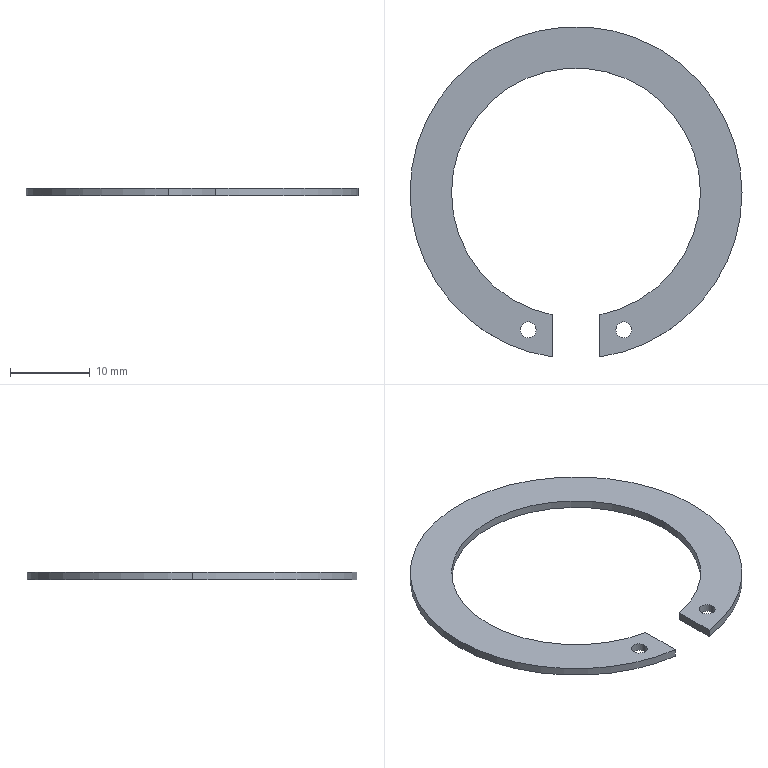Part | STEP file | Mkt rotor clip | 1 solid | 14 faces | box 41.6 x 41.383 x 1 mm | volume 557.011 mm3 | cylinder 10 | plane 4 | commonest cylinder face diameters 2 x4 31.2 x3 41.6 x3
STEP:
#1=CARTESIAN_POINT('',(0.,0.,0.));
#2=DIRECTION('',(0.,0.,1.));
#3=DIRECTION('',(1.,0.,0.));
#4=AXIS2_PLACEMENT_3D('',#1,#2,#3);
#5=CARTESIAN_POINT('',(5.,-17.2,1.));
#6=VERTEX_POINT('',#5);
#7=CARTESIAN_POINT('',(5.,-17.2,0.));
#8=VERTEX_POINT('',#7);
#9=CARTESIAN_POINT('',(5.,-17.2,1.));
#10=DIRECTION('',(0.,0.,-1.));
#11=VECTOR('',#10,1.);
#12=LINE('',#9,#11);
#13=CARTESIAN_POINT('',(6.,-17.2,1.));
#14=DIRECTION('',(0.,0.,-1.));
#15=DIRECTION('',(-1.,0.,0.));
#16=AXIS2_PLACEMENT_3D('',#13,#14,#15);
#17=CYLINDRICAL_SURFACE('',#16,1.);
#18=CARTESIAN_POINT('',(6.283,0.));
#19=DIRECTION('',(0.,1.));
#20=VECTOR('',#19,1.);
#21=LINE('',#18,#20);
#22=(GEOMETRIC_REPRESENTATION_CONTEXT(2)PARAMETRIC_REPRESENTATION_CONTEXT()REPRESENTATION_CONTEXT('',''));
#23=DEFINITIONAL_REPRESENTATION('',(#21),#22);
#24=PCURVE('',#17,#23);
#25=CARTESIAN_POINT('',(6.,-17.2,1.));
#26=DIRECTION('',(0.,0.,-1.));
#27=DIRECTION('',(-1.,0.,0.));
#28=AXIS2_PLACEMENT_3D('',#25,#26,#27);
#29=CYLINDRICAL_SURFACE('',#28,1.);
#30=CARTESIAN_POINT('',(0.,0.));
#31=DIRECTION('',(0.,1.));
#32=VECTOR('',#31,1.);
#33=LINE('',#30,#32);
#34=(GEOMETRIC_REPRESENTATION_CONTEXT(2)PARAMETRIC_REPRESENTATION_CONTEXT()REPRESENTATION_CONTEXT('',''));
#35=DEFINITIONAL_REPRESENTATION('',(#33),#34);
#36=PCURVE('',#29,#35);
#37=SURFACE_CURVE('',#12,(#24,#36),.PCURVE_S1.);
#38=EDGE_CURVE('',#6,#8,#37,.T.);
#39=ORIENTED_EDGE('',*,*,#38,.T.);
#40=CARTESIAN_POINT('',(7.,-17.2,0.));
#41=VERTEX_POINT('',#40);
#42=CARTESIAN_POINT('',(6.,-17.2,0.));
#43=DIRECTION('',(0.,0.,-1.));
#44=DIRECTION('',(-1.,0.,0.));
#45=AXIS2_PLACEMENT_3D('',#42,#43,#44);
#46=CIRCLE('',#45,1.);
#47=CARTESIAN_POINT('',(0.,1.));
#48=DIRECTION('',(1.,0.));
#49=VECTOR('',#48,1.);
#50=LINE('',#47,#49);
#51=(GEOMETRIC_REPRESENTATION_CONTEXT(2)PARAMETRIC_REPRESENTATION_CONTEXT()REPRESENTATION_CONTEXT('',''));
#52=DEFINITIONAL_REPRESENTATION('',(#50),#51);
#53=PCURVE('',#17,#52);
#54=CARTESIAN_POINT('',(0.,0.,0.));
#55=DIRECTION('',(0.,0.,1.));
#56=DIRECTION('',(1.,0.,0.));
#57=AXIS2_PLACEMENT_3D('',#54,#55,#56);
#58=PLANE('',#57);
#59=CARTESIAN_POINT('',(5.,-17.2));
#60=CARTESIAN_POINT('',(5.,-15.468));
#61=CARTESIAN_POINT('',(6.5,-16.334));
#62=CARTESIAN_POINT('',(8.,-17.2));
#63=CARTESIAN_POINT('',(6.5,-18.066));
#64=CARTESIAN_POINT('',(5.,-18.932));
#65=CARTESIAN_POINT('',(5.,-17.2));
#66=(BOUNDED_CURVE()B_SPLINE_CURVE(2,(#59,#60,#61,#62,#63,#64,#65),.UNSPECIFIED.,.T.,.F.)B_SPLINE_CURVE_WITH_KNOTS((1,2,2,2,2,1),(-2.094,0.,2.094,4.189,6.283,8.378),.UNSPECIFIED.)CURVE()GEOMETRIC_REPRESENTATION_ITEM()RATIONAL_B_SPLINE_CURVE((1.,0.5,1.,0.5,1.,0.5,1.))REPRESENTATION_ITEM(''));
#67=(GEOMETRIC_REPRESENTATION_CONTEXT(2)PARAMETRIC_REPRESENTATION_CONTEXT()REPRESENTATION_CONTEXT('',''));
#68=DEFINITIONAL_REPRESENTATION('',(#66),#67);
#69=PCURVE('',#58,#68);
#70=SURFACE_CURVE('',#46,(#53,#69),.PCURVE_S1.);
#71=EDGE_CURVE('',#41,#8,#70,.T.);
#72=ORIENTED_EDGE('',*,*,#71,.F.);
#73=CARTESIAN_POINT('',(7.,-17.2,1.));
#74=VERTEX_POINT('',#73);
#75=CARTESIAN_POINT('',(7.,-17.2,1.));
#76=DIRECTION('',(0.,0.,-1.));
#77=VECTOR('',#76,1.);
#78=LINE('',#75,#77);
#79=CARTESIAN_POINT('',(3.142,0.));
#80=DIRECTION('',(0.,1.));
#81=VECTOR('',#80,1.);
#82=LINE('',#79,#81);
#83=(GEOMETRIC_REPRESENTATION_CONTEXT(2)PARAMETRIC_REPRESENTATION_CONTEXT()REPRESENTATION_CONTEXT('',''));
#84=DEFINITIONAL_REPRESENTATION('',(#82),#83);
#85=PCURVE('',#17,#84);
#86=CARTESIAN_POINT('',(3.142,0.));
#87=DIRECTION('',(0.,1.));
#88=VECTOR('',#87,1.);
#89=LINE('',#86,#88);
#90=(GEOMETRIC_REPRESENTATION_CONTEXT(2)PARAMETRIC_REPRESENTATION_CONTEXT()REPRESENTATION_CONTEXT('',''));
#91=DEFINITIONAL_REPRESENTATION('',(#89),#90);
#92=PCURVE('',#29,#91);
#93=SURFACE_CURVE('',#78,(#85,#92),.PCURVE_S1.);
#94=EDGE_CURVE('',#74,#41,#93,.T.);
#95=ORIENTED_EDGE('',*,*,#94,.F.);
#96=CARTESIAN_POINT('',(6.,-17.2,1.));
#97=DIRECTION('',(0.,0.,-1.));
#98=DIRECTION('',(-1.,0.,0.));
#99=AXIS2_PLACEMENT_3D('',#96,#97,#98);
#100=CIRCLE('',#99,1.);
#101=CARTESIAN_POINT('',(0.,0.));
#102=DIRECTION('',(1.,0.));
#103=VECTOR('',#102,1.);
#104=LINE('',#101,#103);
#105=(GEOMETRIC_REPRESENTATION_CONTEXT(2)PARAMETRIC_REPRESENTATION_CONTEXT()REPRESENTATION_CONTEXT('',''));
#106=DEFINITIONAL_REPRESENTATION('',(#104),#105);
#107=PCURVE('',#17,#106);
#108=CARTESIAN_POINT('',(0.,0.,1.));
#109=DIRECTION('',(0.,0.,1.));
#110=DIRECTION('',(1.,0.,0.));
#111=AXIS2_PLACEMENT_3D('',#108,#109,#110);
#112=PLANE('',#111);
#113=CARTESIAN_POINT('',(5.,-17.2));
#114=CARTESIAN_POINT('',(5.,-15.468));
#115=CARTESIAN_POINT('',(6.5,-16.334));
#116=CARTESIAN_POINT('',(8.,-17.2));
#117=CARTESIAN_POINT('',(6.5,-18.066));
#118=CARTESIAN_POINT('',(5.,-18.932));
#119=CARTESIAN_POINT('',(5.,-17.2));
#120=(BOUNDED_CURVE()B_SPLINE_CURVE(2,(#113,#114,#115,#116,#117,#118,#119),.UNSPECIFIED.,.T.,.F.)B_SPLINE_CURVE_WITH_KNOTS((1,2,2,2,2,1),(-2.094,0.,2.094,4.189,6.283,8.378),.UNSPECIFIED.)CURVE()GEOMETRIC_REPRESENTATION_ITEM()RATIONAL_B_SPLINE_CURVE((1.,0.5,1.,0.5,1.,0.5,1.))REPRESENTATION_ITEM(''));
#121=(GEOMETRIC_REPRESENTATION_CONTEXT(2)PARAMETRIC_REPRESENTATION_CONTEXT()REPRESENTATION_CONTEXT('',''));
#122=DEFINITIONAL_REPRESENTATION('',(#120),#121);
#123=PCURVE('',#112,#122);
#124=SURFACE_CURVE('',#100,(#107,#123),.PCURVE_S1.);
#125=EDGE_CURVE('',#74,#6,#124,.T.);
#126=ORIENTED_EDGE('',*,*,#125,.T.);
#127=EDGE_LOOP('',(#39,#72,#95,#126));
#128=FACE_BOUND('',#127,.F.);
#129=ADVANCED_FACE('',(#128),#17,.F.);
#130=CARTESIAN_POINT('',(3.,-15.309,0.));
#131=VERTEX_POINT('',#130);
#132=CARTESIAN_POINT('',(3.,-15.309,1.));
#133=VERTEX_POINT('',#132);
#134=CARTESIAN_POINT('',(3.,-15.309,1.));
#135=DIRECTION('',(0.,0.,1.));
#136=VECTOR('',#135,1.);
#137=LINE('',#134,#136);
#138=CARTESIAN_POINT('',(0.,0.,1.));
#139=DIRECTION('',(0.,0.,-1.));
#140=DIRECTION('',(-1.,0.,0.));
#141=AXIS2_PLACEMENT_3D('',#138,#139,#140);
#142=CYLINDRICAL_SURFACE('',#141,15.6);
#143=CARTESIAN_POINT('',(4.519,0.));
#144=DIRECTION('',(0.,-1.));
#145=VECTOR('',#144,1.);
#146=LINE('',#143,#145);
#147=(GEOMETRIC_REPRESENTATION_CONTEXT(2)PARAMETRIC_REPRESENTATION_CONTEXT()REPRESENTATION_CONTEXT('',''));
#148=DEFINITIONAL_REPRESENTATION('',(#146),#147);
#149=PCURVE('',#142,#148);
#150=CARTESIAN_POINT('',(3.,-15.309,1.));
#151=DIRECTION('',(1.,0.,0.));
#152=DIRECTION('',(0.,0.,-1.));
#153=AXIS2_PLACEMENT_3D('',#150,#151,#152);
#154=PLANE('',#153);
#155=CARTESIAN_POINT('',(0.,0.));
#156=DIRECTION('',(-1.,0.));
#157=VECTOR('',#156,1.);
#158=LINE('',#155,#157);
#159=(GEOMETRIC_REPRESENTATION_CONTEXT(2)PARAMETRIC_REPRESENTATION_CONTEXT()REPRESENTATION_CONTEXT('',''));
#160=DEFINITIONAL_REPRESENTATION('',(#158),#159);
#161=PCURVE('',#154,#160);
#162=SURFACE_CURVE('',#137,(#149,#161),.PCURVE_S1.);
#163=EDGE_CURVE('',#131,#133,#162,.T.);
#164=ORIENTED_EDGE('',*,*,#163,.F.);
#165=CARTESIAN_POINT('',(15.6,0.,0.));
#166=VERTEX_POINT('',#165);
#167=CARTESIAN_POINT('',(0.,0.,0.));
#168=DIRECTION('',(0.,0.,-1.));
#169=DIRECTION('',(-1.,0.,0.));
#170=AXIS2_PLACEMENT_3D('',#167,#168,#169);
#171=CIRCLE('',#170,15.6);
#172=CARTESIAN_POINT('',(0.,1.));
#173=DIRECTION('',(1.,0.));
#174=VECTOR('',#173,1.);
#175=LINE('',#172,#174);
#176=(GEOMETRIC_REPRESENTATION_CONTEXT(2)PARAMETRIC_REPRESENTATION_CONTEXT()REPRESENTATION_CONTEXT('',''));
#177=DEFINITIONAL_REPRESENTATION('',(#175),#176);
#178=PCURVE('',#142,#177);
#179=CARTESIAN_POINT('',(-15.6,0.));
#180=CARTESIAN_POINT('',(-15.6,27.02));
#181=CARTESIAN_POINT('',(7.8,13.51));
#182=CARTESIAN_POINT('',(31.2,0.));
#183=CARTESIAN_POINT('',(7.8,-13.51));
#184=CARTESIAN_POINT('',(-15.6,-27.02));
#185=CARTESIAN_POINT('',(-15.6,0.));
#186=(BOUNDED_CURVE()B_SPLINE_CURVE(2,(#179,#180,#181,#182,#183,#184,#185),.UNSPECIFIED.,.T.,.F.)B_SPLINE_CURVE_WITH_KNOTS((1,2,2,2,2,1),(-2.094,0.,2.094,4.189,6.283,8.378),.UNSPECIFIED.)CURVE()GEOMETRIC_REPRESENTATION_ITEM()RATIONAL_B_SPLINE_CURVE((1.,0.5,1.,0.5,1.,0.5,1.))REPRESENTATION_ITEM(''));
#187=(GEOMETRIC_REPRESENTATION_CONTEXT(2)PARAMETRIC_REPRESENTATION_CONTEXT()REPRESENTATION_CONTEXT('',''));
#188=DEFINITIONAL_REPRESENTATION('',(#186),#187);
#189=PCURVE('',#58,#188);
#190=SURFACE_CURVE('',#171,(#178,#189),.PCURVE_S1.);
#191=EDGE_CURVE('',#166,#131,#190,.T.);
#192=ORIENTED_EDGE('',*,*,#191,.F.);
#193=CARTESIAN_POINT('',(15.6,0.,1.));
#194=VERTEX_POINT('',#193);
#195=CARTESIAN_POINT('',(15.6,0.,1.));
#196=DIRECTION('',(0.,0.,-1.));
#197=VECTOR('',#196,1.);
#198=LINE('',#195,#197);
#199=CARTESIAN_POINT('',(3.142,0.));
#200=DIRECTION('',(0.,1.));
#201=VECTOR('',#200,1.);
#202=LINE('',#199,#201);
#203=(GEOMETRIC_REPRESENTATION_CONTEXT(2)PARAMETRIC_REPRESENTATION_CONTEXT()REPRESENTATION_CONTEXT('',''));
#204=DEFINITIONAL_REPRESENTATION('',(#202),#203);
#205=PCURVE('',#142,#204);
#206=CARTESIAN_POINT('',(0.,0.,1.));
#207=DIRECTION('',(0.,0.,-1.));
#208=DIRECTION('',(-1.,0.,0.));
#209=AXIS2_PLACEMENT_3D('',#206,#207,#208);
#210=CYLINDRICAL_SURFACE('',#209,15.6);
#211=CARTESIAN_POINT('',(3.142,0.));
#212=DIRECTION('',(0.,1.));
#213=VECTOR('',#212,1.);
#214=LINE('',#211,#213);
#215=(GEOMETRIC_REPRESENTATION_CONTEXT(2)PARAMETRIC_REPRESENTATION_CONTEXT()REPRESENTATION_CONTEXT('',''));
#216=DEFINITIONAL_REPRESENTATION('',(#214),#215);
#217=PCURVE('',#210,#216);
#218=SURFACE_CURVE('',#198,(#205,#217),.PCURVE_S1.);
#219=EDGE_CURVE('',#194,#166,#218,.T.);
#220=ORIENTED_EDGE('',*,*,#219,.F.);
#221=CARTESIAN_POINT('',(0.,0.,1.));
#222=DIRECTION('',(0.,0.,-1.));
#223=DIRECTION('',(-1.,0.,0.));
#224=AXIS2_PLACEMENT_3D('',#221,#222,#223);
#225=CIRCLE('',#224,15.6);
#226=CARTESIAN_POINT('',(0.,0.));
#227=DIRECTION('',(1.,0.));
#228=VECTOR('',#227,1.);
#229=LINE('',#226,#228);
#230=(GEOMETRIC_REPRESENTATION_CONTEXT(2)PARAMETRIC_REPRESENTATION_CONTEXT()REPRESENTATION_CONTEXT('',''));
#231=DEFINITIONAL_REPRESENTATION('',(#229),#230);
#232=PCURVE('',#142,#231);
#233=CARTESIAN_POINT('',(-15.6,0.));
#234=CARTESIAN_POINT('',(-15.6,27.02));
#235=CARTESIAN_POINT('',(7.8,13.51));
#236=CARTESIAN_POINT('',(31.2,0.));
#237=CARTESIAN_POINT('',(7.8,-13.51));
#238=CARTESIAN_POINT('',(-15.6,-27.02));
#239=CARTESIAN_POINT('',(-15.6,0.));
#240=(BOUNDED_CURVE()B_SPLINE_CURVE(2,(#233,#234,#235,#236,#237,#238,#239),.UNSPECIFIED.,.T.,.F.)B_SPLINE_CURVE_WITH_KNOTS((1,2,2,2,2,1),(-2.094,0.,2.094,4.189,6.283,8.378),.UNSPECIFIED.)CURVE()GEOMETRIC_REPRESENTATION_ITEM()RATIONAL_B_SPLINE_CURVE((1.,0.5,1.,0.5,1.,0.5,1.))REPRESENTATION_ITEM(''));
#241=(GEOMETRIC_REPRESENTATION_CONTEXT(2)PARAMETRIC_REPRESENTATION_CONTEXT()REPRESENTATION_CONTEXT('',''));
#242=DEFINITIONAL_REPRESENTATION('',(#240),#241);
#243=PCURVE('',#112,#242);
#244=SURFACE_CURVE('',#225,(#232,#243),.PCURVE_S1.);
#245=EDGE_CURVE('',#194,#133,#244,.T.);
#246=ORIENTED_EDGE('',*,*,#245,.T.);
#247=EDGE_LOOP('',(#164,#192,#220,#246));
#248=FACE_BOUND('',#247,.F.);
#249=ADVANCED_FACE('',(#248),#142,.F.);
#250=CARTESIAN_POINT('',(-15.6,0.,0.));
#251=VERTEX_POINT('',#250);
#252=CARTESIAN_POINT('',(0.,0.,0.));
#253=DIRECTION('',(0.,0.,-1.));
#254=DIRECTION('',(-1.,0.,0.));
#255=AXIS2_PLACEMENT_3D('',#252,#253,#254);
#256=CIRCLE('',#255,15.6);
#257=CARTESIAN_POINT('',(0.,1.));
#258=DIRECTION('',(1.,0.));
#259=VECTOR('',#258,1.);
#260=LINE('',#257,#259);
#261=(GEOMETRIC_REPRESENTATION_CONTEXT(2)PARAMETRIC_REPRESENTATION_CONTEXT()REPRESENTATION_CONTEXT('',''));
#262=DEFINITIONAL_REPRESENTATION('',(#260),#261);
#263=PCURVE('',#210,#262);
#264=CARTESIAN_POINT('',(-15.6,0.));
#265=CARTESIAN_POINT('',(-15.6,27.02));
#266=CARTESIAN_POINT('',(7.8,13.51));
#267=CARTESIAN_POINT('',(31.2,0.));
#268=CARTESIAN_POINT('',(7.8,-13.51));
#269=CARTESIAN_POINT('',(-15.6,-27.02));
#270=CARTESIAN_POINT('',(-15.6,0.));
#271=(BOUNDED_CURVE()B_SPLINE_CURVE(2,(#264,#265,#266,#267,#268,#269,#270),.UNSPECIFIED.,.T.,.F.)B_SPLINE_CURVE_WITH_KNOTS((1,2,2,2,2,1),(-2.094,0.,2.094,4.189,6.283,8.378),.UNSPECIFIED.)CURVE()GEOMETRIC_REPRESENTATION_ITEM()RATIONAL_B_SPLINE_CURVE((1.,0.5,1.,0.5,1.,0.5,1.))REPRESENTATION_ITEM(''));
#272=(GEOMETRIC_REPRESENTATION_CONTEXT(2)PARAMETRIC_REPRESENTATION_CONTEXT()REPRESENTATION_CONTEXT('',''));
#273=DEFINITIONAL_REPRESENTATION('',(#271),#272);
#274=PCURVE('',#58,#273);
#275=SURFACE_CURVE('',#256,(#263,#274),.PCURVE_S1.);
#276=EDGE_CURVE('',#251,#166,#275,.T.);
#277=ORIENTED_EDGE('',*,*,#276,.F.);
#278=CARTESIAN_POINT('',(-15.6,0.,1.));
#279=VERTEX_POINT('',#278);
#280=CARTESIAN_POINT('',(-15.6,0.,1.));
#281=DIRECTION('',(0.,0.,-1.));
#282=VECTOR('',#281,1.);
#283=LINE('',#280,#282);
#284=CARTESIAN_POINT('',(0.,0.));
#285=DIRECTION('',(0.,1.));
#286=VECTOR('',#285,1.);
#287=LINE('',#284,#286);
#288=(GEOMETRIC_REPRESENTATION_CONTEXT(2)PARAMETRIC_REPRESENTATION_CONTEXT()REPRESENTATION_CONTEXT('',''));
#289=DEFINITIONAL_REPRESENTATION('',(#287),#288);
#290=PCURVE('',#210,#289);
#291=CARTESIAN_POINT('',(0.,0.,1.));
#292=DIRECTION('',(0.,0.,-1.));
#293=DIRECTION('',(-1.,0.,0.));
#294=AXIS2_PLACEMENT_3D('',#291,#292,#293);
#295=CYLINDRICAL_SURFACE('',#294,15.6);
#296=CARTESIAN_POINT('',(6.283,0.));
#297=DIRECTION('',(0.,1.));
#298=VECTOR('',#297,1.);
#299=LINE('',#296,#298);
#300=(GEOMETRIC_REPRESENTATION_CONTEXT(2)PARAMETRIC_REPRESENTATION_CONTEXT()REPRESENTATION_CONTEXT('',''));
#301=DEFINITIONAL_REPRESENTATION('',(#299),#300);
#302=PCURVE('',#295,#301);
#303=SURFACE_CURVE('',#283,(#290,#302),.PCURVE_S1.);
#304=EDGE_CURVE('',#279,#251,#303,.T.);
#305=ORIENTED_EDGE('',*,*,#304,.F.);
#306=CARTESIAN_POINT('',(0.,0.,1.));
#307=DIRECTION('',(0.,0.,-1.));
#308=DIRECTION('',(-1.,0.,0.));
#309=AXIS2_PLACEMENT_3D('',#306,#307,#308);
#310=CIRCLE('',#309,15.6);
#311=CARTESIAN_POINT('',(0.,0.));
#312=DIRECTION('',(1.,0.));
#313=VECTOR('',#312,1.);
#314=LINE('',#311,#313);
#315=(GEOMETRIC_REPRESENTATION_CONTEXT(2)PARAMETRIC_REPRESENTATION_CONTEXT()REPRESENTATION_CONTEXT('',''));
#316=DEFINITIONAL_REPRESENTATION('',(#314),#315);
#317=PCURVE('',#210,#316);
#318=CARTESIAN_POINT('',(-15.6,0.));
#319=CARTESIAN_POINT('',(-15.6,27.02));
#320=CARTESIAN_POINT('',(7.8,13.51));
#321=CARTESIAN_POINT('',(31.2,0.));
#322=CARTESIAN_POINT('',(7.8,-13.51));
#323=CARTESIAN_POINT('',(-15.6,-27.02));
#324=CARTESIAN_POINT('',(-15.6,0.));
#325=(BOUNDED_CURVE()B_SPLINE_CURVE(2,(#318,#319,#320,#321,#322,#323,#324),.UNSPECIFIED.,.T.,.F.)B_SPLINE_CURVE_WITH_KNOTS((1,2,2,2,2,1),(-2.094,0.,2.094,4.189,6.283,8.378),.UNSPECIFIED.)CURVE()GEOMETRIC_REPRESENTATION_ITEM()RATIONAL_B_SPLINE_CURVE((1.,0.5,1.,0.5,1.,0.5,1.))REPRESENTATION_ITEM(''));
#326=(GEOMETRIC_REPRESENTATION_CONTEXT(2)PARAMETRIC_REPRESENTATION_CONTEXT()REPRESENTATION_CONTEXT('',''));
#327=DEFINITIONAL_REPRESENTATION('',(#325),#326);
#328=PCURVE('',#112,#327);
#329=SURFACE_CURVE('',#310,(#317,#328),.PCURVE_S1.);
#330=EDGE_CURVE('',#279,#194,#329,.T.);
#331=ORIENTED_EDGE('',*,*,#330,.T.);
#332=ORIENTED_EDGE('',*,*,#219,.T.);
#333=EDGE_LOOP('',(#277,#305,#331,#332));
#334=FACE_BOUND('',#333,.F.);
#335=ADVANCED_FACE('',(#334),#210,.F.);
#336=CARTESIAN_POINT('',(-20.8,0.,1.));
#337=VERTEX_POINT('',#336);
#338=CARTESIAN_POINT('',(20.8,0.,1.));
#339=VERTEX_POINT('',#338);
#340=CARTESIAN_POINT('',(0.,0.,1.));
#341=DIRECTION('',(0.,0.,-1.));
#342=DIRECTION('',(-1.,0.,0.));
#343=AXIS2_PLACEMENT_3D('',#340,#341,#342);
#344=CIRCLE('',#343,20.8);
#345=CARTESIAN_POINT('',(0.,0.,1.));
#346=DIRECTION('',(0.,0.,-1.));
#347=DIRECTION('',(-1.,0.,0.));
#348=AXIS2_PLACEMENT_3D('',#345,#346,#347);
#349=CYLINDRICAL_SURFACE('',#348,20.8);
#350=CARTESIAN_POINT('',(0.,0.));
#351=DIRECTION('',(1.,0.));
#352=VECTOR('',#351,1.);
#353=LINE('',#350,#352);
#354=(GEOMETRIC_REPRESENTATION_CONTEXT(2)PARAMETRIC_REPRESENTATION_CONTEXT()REPRESENTATION_CONTEXT('',''));
#355=DEFINITIONAL_REPRESENTATION('',(#353),#354);
#356=PCURVE('',#349,#355);
#357=CARTESIAN_POINT('',(-20.8,0.));
#358=CARTESIAN_POINT('',(-20.8,36.027));
#359=CARTESIAN_POINT('',(10.4,18.013));
#360=CARTESIAN_POINT('',(41.6,0.));
#361=CARTESIAN_POINT('',(10.4,-18.013));
#362=CARTESIAN_POINT('',(-20.8,-36.027));
#363=CARTESIAN_POINT('',(-20.8,0.));
#364=(BOUNDED_CURVE()B_SPLINE_CURVE(2,(#357,#358,#359,#360,#361,#362,#363),.UNSPECIFIED.,.T.,.F.)B_SPLINE_CURVE_WITH_KNOTS((1,2,2,2,2,1),(-2.094,0.,2.094,4.189,6.283,8.378),.UNSPECIFIED.)CURVE()GEOMETRIC_REPRESENTATION_ITEM()RATIONAL_B_SPLINE_CURVE((1.,0.5,1.,0.5,1.,0.5,1.))REPRESENTATION_ITEM(''));
#365=(GEOMETRIC_REPRESENTATION_CONTEXT(2)PARAMETRIC_REPRESENTATION_CONTEXT()REPRESENTATION_CONTEXT('',''));
#366=DEFINITIONAL_REPRESENTATION('',(#364),#365);
#367=PCURVE('',#112,#366);
#368=SURFACE_CURVE('',#344,(#356,#367),.PCURVE_S1.);
#369=EDGE_CURVE('',#337,#339,#368,.T.);
#370=ORIENTED_EDGE('',*,*,#369,.T.);
#371=CARTESIAN_POINT('',(20.8,0.,0.));
#372=VERTEX_POINT('',#371);
#373=CARTESIAN_POINT('',(20.8,0.,1.));
#374=DIRECTION('',(0.,0.,-1.));
#375=VECTOR('',#374,1.);
#376=LINE('',#373,#375);
#377=CARTESIAN_POINT('',(3.142,0.));
#378=DIRECTION('',(0.,1.));
#379=VECTOR('',#378,1.);
#380=LINE('',#377,#379);
#381=(GEOMETRIC_REPRESENTATION_CONTEXT(2)PARAMETRIC_REPRESENTATION_CONTEXT()REPRESENTATION_CONTEXT('',''));
#382=DEFINITIONAL_REPRESENTATION('',(#380),#381);
#383=PCURVE('',#349,#382);
#384=CARTESIAN_POINT('',(0.,0.,1.));
#385=DIRECTION('',(0.,0.,-1.));
#386=DIRECTION('',(-1.,0.,0.));
#387=AXIS2_PLACEMENT_3D('',#384,#385,#386);
#388=CYLINDRICAL_SURFACE('',#387,20.8);
#389=CARTESIAN_POINT('',(3.142,0.));
#390=DIRECTION('',(0.,1.));
#391=VECTOR('',#390,1.);
#392=LINE('',#389,#391);
#393=(GEOMETRIC_REPRESENTATION_CONTEXT(2)PARAMETRIC_REPRESENTATION_CONTEXT()REPRESENTATION_CONTEXT('',''));
#394=DEFINITIONAL_REPRESENTATION('',(#392),#393);
#395=PCURVE('',#388,#394);
#396=SURFACE_CURVE('',#376,(#383,#395),.PCURVE_S1.);
#397=EDGE_CURVE('',#339,#372,#396,.T.);
#398=ORIENTED_EDGE('',*,*,#397,.T.);
#399=CARTESIAN_POINT('',(-20.8,0.,0.));
#400=VERTEX_POINT('',#399);
#401=CARTESIAN_POINT('',(0.,0.,0.));
#402=DIRECTION('',(0.,0.,1.));
#403=DIRECTION('',(-1.,0.,0.));
#404=AXIS2_PLACEMENT_3D('',#401,#402,#403);
#405=CIRCLE('',#404,20.8);
#406=CARTESIAN_POINT('',(6.283,1.));
#407=DIRECTION('',(-1.,0.));
#408=VECTOR('',#407,1.);
#409=LINE('',#406,#408);
#410=(GEOMETRIC_REPRESENTATION_CONTEXT(2)PARAMETRIC_REPRESENTATION_CONTEXT()REPRESENTATION_CONTEXT('',''));
#411=DEFINITIONAL_REPRESENTATION('',(#409),#410);
#412=PCURVE('',#349,#411);
#413=CARTESIAN_POINT('',(0.,0.));
#414=DIRECTION('',(-1.,0.));
#415=AXIS2_PLACEMENT_2D('',#413,#414);
#416=CIRCLE('',#415,20.8);
#417=(GEOMETRIC_REPRESENTATION_CONTEXT(2)PARAMETRIC_REPRESENTATION_CONTEXT()REPRESENTATION_CONTEXT('',''));
#418=DEFINITIONAL_REPRESENTATION('',(#416),#417);
#419=PCURVE('',#58,#418);
#420=SURFACE_CURVE('',#405,(#412,#419),.PCURVE_S1.);
#421=EDGE_CURVE('',#372,#400,#420,.T.);
#422=ORIENTED_EDGE('',*,*,#421,.T.);
#423=CARTESIAN_POINT('',(-20.8,0.,1.));
#424=DIRECTION('',(0.,0.,-1.));
#425=VECTOR('',#424,1.);
#426=LINE('',#423,#425);
#427=CARTESIAN_POINT('',(0.,0.));
#428=DIRECTION('',(0.,1.));
#429=VECTOR('',#428,1.);
#430=LINE('',#427,#429);
#431=(GEOMETRIC_REPRESENTATION_CONTEXT(2)PARAMETRIC_REPRESENTATION_CONTEXT()REPRESENTATION_CONTEXT('',''));
#432=DEFINITIONAL_REPRESENTATION('',(#430),#431);
#433=PCURVE('',#349,#432);
#434=CARTESIAN_POINT('',(0.,0.,1.));
#435=DIRECTION('',(0.,0.,-1.));
#436=DIRECTION('',(-1.,0.,0.));
#437=AXIS2_PLACEMENT_3D('',#434,#435,#436);
#438=CYLINDRICAL_SURFACE('',#437,20.8);
#439=CARTESIAN_POINT('',(6.283,0.));
#440=DIRECTION('',(0.,1.));
#441=VECTOR('',#440,1.);
#442=LINE('',#439,#441);
#443=(GEOMETRIC_REPRESENTATION_CONTEXT(2)PARAMETRIC_REPRESENTATION_CONTEXT()REPRESENTATION_CONTEXT('',''));
#444=DEFINITIONAL_REPRESENTATION('',(#442),#443);
#445=PCURVE('',#438,#444);
#446=SURFACE_CURVE('',#426,(#433,#445),.PCURVE_S1.);
#447=EDGE_CURVE('',#337,#400,#446,.T.);
#448=ORIENTED_EDGE('',*,*,#447,.F.);
#449=EDGE_LOOP('',(#370,#398,#422,#448));
#450=FACE_BOUND('',#449,.T.);
#451=ADVANCED_FACE('',(#450),#349,.T.);
#452=CARTESIAN_POINT('',(-3.,-20.583,1.));
#453=VERTEX_POINT('',#452);
#454=CARTESIAN_POINT('',(0.,0.,1.));
#455=DIRECTION('',(0.,0.,-1.));
#456=DIRECTION('',(-1.,0.,0.));
#457=AXIS2_PLACEMENT_3D('',#454,#455,#456);
#458=CIRCLE('',#457,20.8);
#459=CARTESIAN_POINT('',(0.,0.));
#460=DIRECTION('',(1.,0.));
#461=VECTOR('',#460,1.);
#462=LINE('',#459,#461);
#463=(GEOMETRIC_REPRESENTATION_CONTEXT(2)PARAMETRIC_REPRESENTATION_CONTEXT()REPRESENTATION_CONTEXT('',''));
#464=DEFINITIONAL_REPRESENTATION('',(#462),#463);
#465=PCURVE('',#438,#464);
#466=CARTESIAN_POINT('',(-20.8,0.));
#467=CARTESIAN_POINT('',(-20.8,36.027));
#468=CARTESIAN_POINT('',(10.4,18.013));
#469=CARTESIAN_POINT('',(41.6,0.));
#470=CARTESIAN_POINT('',(10.4,-18.013));
#471=CARTESIAN_POINT('',(-20.8,-36.027));
#472=CARTESIAN_POINT('',(-20.8,0.));
#473=(BOUNDED_CURVE()B_SPLINE_CURVE(2,(#466,#467,#468,#469,#470,#471,#472),.UNSPECIFIED.,.T.,.F.)B_SPLINE_CURVE_WITH_KNOTS((1,2,2,2,2,1),(-2.094,0.,2.094,4.189,6.283,8.378),.UNSPECIFIED.)CURVE()GEOMETRIC_REPRESENTATION_ITEM()RATIONAL_B_SPLINE_CURVE((1.,0.5,1.,0.5,1.,0.5,1.))REPRESENTATION_ITEM(''));
#474=(GEOMETRIC_REPRESENTATION_CONTEXT(2)PARAMETRIC_REPRESENTATION_CONTEXT()REPRESENTATION_CONTEXT('',''));
#475=DEFINITIONAL_REPRESENTATION('',(#473),#474);
#476=PCURVE('',#112,#475);
#477=SURFACE_CURVE('',#458,(#465,#476),.PCURVE_S1.);
#478=EDGE_CURVE('',#453,#337,#477,.T.);
#479=ORIENTED_EDGE('',*,*,#478,.T.);
#480=ORIENTED_EDGE('',*,*,#447,.T.);
#481=CARTESIAN_POINT('',(-3.,-20.583,0.));
#482=VERTEX_POINT('',#481);
#483=CARTESIAN_POINT('',(0.,0.,0.));
#484=DIRECTION('',(0.,0.,1.));
#485=DIRECTION('',(-1.,0.,0.));
#486=AXIS2_PLACEMENT_3D('',#483,#484,#485);
#487=CIRCLE('',#486,20.8);
#488=CARTESIAN_POINT('',(6.283,1.));
#489=DIRECTION('',(-1.,0.));
#490=VECTOR('',#489,1.);
#491=LINE('',#488,#490);
#492=(GEOMETRIC_REPRESENTATION_CONTEXT(2)PARAMETRIC_REPRESENTATION_CONTEXT()REPRESENTATION_CONTEXT('',''));
#493=DEFINITIONAL_REPRESENTATION('',(#491),#492);
#494=PCURVE('',#438,#493);
#495=CARTESIAN_POINT('',(0.,0.));
#496=DIRECTION('',(-1.,0.));
#497=AXIS2_PLACEMENT_2D('',#495,#496);
#498=CIRCLE('',#497,20.8);
#499=(GEOMETRIC_REPRESENTATION_CONTEXT(2)PARAMETRIC_REPRESENTATION_CONTEXT()REPRESENTATION_CONTEXT('',''));
#500=DEFINITIONAL_REPRESENTATION('',(#498),#499);
#501=PCURVE('',#58,#500);
#502=SURFACE_CURVE('',#487,(#494,#501),.PCURVE_S1.);
#503=EDGE_CURVE('',#400,#482,#502,.T.);
#504=ORIENTED_EDGE('',*,*,#503,.T.);
#505=CARTESIAN_POINT('',(-3.,-20.583,1.));
#506=DIRECTION('',(0.,0.,1.));
#507=VECTOR('',#506,1.);
#508=LINE('',#505,#507);
#509=CARTESIAN_POINT('',(4.857,0.));
#510=DIRECTION('',(0.,-1.));
#511=VECTOR('',#510,1.);
#512=LINE('',#509,#511);
#513=(GEOMETRIC_REPRESENTATION_CONTEXT(2)PARAMETRIC_REPRESENTATION_CONTEXT()REPRESENTATION_CONTEXT('',''));
#514=DEFINITIONAL_REPRESENTATION('',(#512),#513);
#515=PCURVE('',#438,#514);
#516=CARTESIAN_POINT('',(-3.,-15.309,1.));
#517=DIRECTION('',(-1.,0.,0.));
#518=DIRECTION('',(0.,0.,1.));
#519=AXIS2_PLACEMENT_3D('',#516,#517,#518);
#520=PLANE('',#519);
#521=CARTESIAN_POINT('',(0.,-5.274));
#522=DIRECTION('',(1.,0.));
#523=VECTOR('',#522,1.);
#524=LINE('',#521,#523);
#525=(GEOMETRIC_REPRESENTATION_CONTEXT(2)PARAMETRIC_REPRESENTATION_CONTEXT()REPRESENTATION_CONTEXT('',''));
#526=DEFINITIONAL_REPRESENTATION('',(#524),#525);
#527=PCURVE('',#520,#526);
#528=SURFACE_CURVE('',#508,(#515,#527),.PCURVE_S1.);
#529=EDGE_CURVE('',#482,#453,#528,.T.);
#530=ORIENTED_EDGE('',*,*,#529,.T.);
#531=EDGE_LOOP('',(#479,#480,#504,#530));
#532=FACE_BOUND('',#531,.T.);
#533=ADVANCED_FACE('',(#532),#438,.T.);
#534=CARTESIAN_POINT('',(-7.,-17.2,1.));
#535=VERTEX_POINT('',#534);
#536=CARTESIAN_POINT('',(-7.,-17.2,0.));
#537=VERTEX_POINT('',#536);
#538=CARTESIAN_POINT('',(-7.,-17.2,1.));
#539=DIRECTION('',(0.,0.,-1.));
#540=VECTOR('',#539,1.);
#541=LINE('',#538,#540);
#542=CARTESIAN_POINT('',(-6.,-17.2,1.));
#543=DIRECTION('',(0.,0.,-1.));
#544=DIRECTION('',(-1.,0.,0.));
#545=AXIS2_PLACEMENT_3D('',#542,#543,#544);
#546=CYLINDRICAL_SURFACE('',#545,1.);
#547=CARTESIAN_POINT('',(6.283,0.));
#548=DIRECTION('',(0.,1.));
#549=VECTOR('',#548,1.);
#550=LINE('',#547,#549);
#551=(GEOMETRIC_REPRESENTATION_CONTEXT(2)PARAMETRIC_REPRESENTATION_CONTEXT()REPRESENTATION_CONTEXT('',''));
#552=DEFINITIONAL_REPRESENTATION('',(#550),#551);
#553=PCURVE('',#546,#552);
#554=CARTESIAN_POINT('',(-6.,-17.2,1.));
#555=DIRECTION('',(0.,0.,-1.));
#556=DIRECTION('',(-1.,0.,0.));
#557=AXIS2_PLACEMENT_3D('',#554,#555,#556);
#558=CYLINDRICAL_SURFACE('',#557,1.);
#559=CARTESIAN_POINT('',(0.,0.));
#560=DIRECTION('',(0.,1.));
#561=VECTOR('',#560,1.);
#562=LINE('',#559,#561);
#563=(GEOMETRIC_REPRESENTATION_CONTEXT(2)PARAMETRIC_REPRESENTATION_CONTEXT()REPRESENTATION_CONTEXT('',''));
#564=DEFINITIONAL_REPRESENTATION('',(#562),#563);
#565=PCURVE('',#558,#564);
#566=SURFACE_CURVE('',#541,(#553,#565),.PCURVE_S1.);
#567=EDGE_CURVE('',#535,#537,#566,.T.);
#568=ORIENTED_EDGE('',*,*,#567,.T.);
#569=CARTESIAN_POINT('',(-5.,-17.2,0.));
#570=VERTEX_POINT('',#569);
#571=CARTESIAN_POINT('',(-6.,-17.2,0.));
#572=DIRECTION('',(0.,0.,-1.));
#573=DIRECTION('',(-1.,0.,0.));
#574=AXIS2_PLACEMENT_3D('',#571,#572,#573);
#575=CIRCLE('',#574,1.);
#576=CARTESIAN_POINT('',(0.,1.));
#577=DIRECTION('',(1.,0.));
#578=VECTOR('',#577,1.);
#579=LINE('',#576,#578);
#580=(GEOMETRIC_REPRESENTATION_CONTEXT(2)PARAMETRIC_REPRESENTATION_CONTEXT()REPRESENTATION_CONTEXT('',''));
#581=DEFINITIONAL_REPRESENTATION('',(#579),#580);
#582=PCURVE('',#546,#581);
#583=CARTESIAN_POINT('',(-7.,-17.2));
#584=CARTESIAN_POINT('',(-7.,-15.468));
#585=CARTESIAN_POINT('',(-5.5,-16.334));
#586=CARTESIAN_POINT('',(-4.,-17.2));
#587=CARTESIAN_POINT('',(-5.5,-18.066));
#588=CARTESIAN_POINT('',(-7.,-18.932));
#589=CARTESIAN_POINT('',(-7.,-17.2));
#590=(BOUNDED_CURVE()B_SPLINE_CURVE(2,(#583,#584,#585,#586,#587,#588,#589),.UNSPECIFIED.,.T.,.F.)B_SPLINE_CURVE_WITH_KNOTS((1,2,2,2,2,1),(-2.094,0.,2.094,4.189,6.283,8.378),.UNSPECIFIED.)CURVE()GEOMETRIC_REPRESENTATION_ITEM()RATIONAL_B_SPLINE_CURVE((1.,0.5,1.,0.5,1.,0.5,1.))REPRESENTATION_ITEM(''));
#591=(GEOMETRIC_REPRESENTATION_CONTEXT(2)PARAMETRIC_REPRESENTATION_CONTEXT()REPRESENTATION_CONTEXT('',''));
#592=DEFINITIONAL_REPRESENTATION('',(#590),#591);
#593=PCURVE('',#58,#592);
#594=SURFACE_CURVE('',#575,(#582,#593),.PCURVE_S1.);
#595=EDGE_CURVE('',#570,#537,#594,.T.);
#596=ORIENTED_EDGE('',*,*,#595,.F.);
#597=CARTESIAN_POINT('',(-5.,-17.2,1.));
#598=VERTEX_POINT('',#597);
#599=CARTESIAN_POINT('',(-5.,-17.2,1.));
#600=DIRECTION('',(0.,0.,-1.));
#601=VECTOR('',#600,1.);
#602=LINE('',#599,#601);
#603=CARTESIAN_POINT('',(3.142,0.));
#604=DIRECTION('',(0.,1.));
#605=VECTOR('',#604,1.);
#606=LINE('',#603,#605);
#607=(GEOMETRIC_REPRESENTATION_CONTEXT(2)PARAMETRIC_REPRESENTATION_CONTEXT()REPRESENTATION_CONTEXT('',''));
#608=DEFINITIONAL_REPRESENTATION('',(#606),#607);
#609=PCURVE('',#546,#608);
#610=CARTESIAN_POINT('',(3.142,0.));
#611=DIRECTION('',(0.,1.));
#612=VECTOR('',#611,1.);
#613=LINE('',#610,#612);
#614=(GEOMETRIC_REPRESENTATION_CONTEXT(2)PARAMETRIC_REPRESENTATION_CONTEXT()REPRESENTATION_CONTEXT('',''));
#615=DEFINITIONAL_REPRESENTATION('',(#613),#614);
#616=PCURVE('',#558,#615);
#617=SURFACE_CURVE('',#602,(#609,#616),.PCURVE_S1.);
#618=EDGE_CURVE('',#598,#570,#617,.T.);
#619=ORIENTED_EDGE('',*,*,#618,.F.);
#620=CARTESIAN_POINT('',(-6.,-17.2,1.));
#621=DIRECTION('',(0.,0.,-1.));
#622=DIRECTION('',(-1.,0.,0.));
#623=AXIS2_PLACEMENT_3D('',#620,#621,#622);
#624=CIRCLE('',#623,1.);
#625=CARTESIAN_POINT('',(0.,0.));
#626=DIRECTION('',(1.,0.));
#627=VECTOR('',#626,1.);
#628=LINE('',#625,#627);
#629=(GEOMETRIC_REPRESENTATION_CONTEXT(2)PARAMETRIC_REPRESENTATION_CONTEXT()REPRESENTATION_CONTEXT('',''));
#630=DEFINITIONAL_REPRESENTATION('',(#628),#629);
#631=PCURVE('',#546,#630);
#632=CARTESIAN_POINT('',(-7.,-17.2));
#633=CARTESIAN_POINT('',(-7.,-15.468));
#634=CARTESIAN_POINT('',(-5.5,-16.334));
#635=CARTESIAN_POINT('',(-4.,-17.2));
#636=CARTESIAN_POINT('',(-5.5,-18.066));
#637=CARTESIAN_POINT('',(-7.,-18.932));
#638=CARTESIAN_POINT('',(-7.,-17.2));
#639=(BOUNDED_CURVE()B_SPLINE_CURVE(2,(#632,#633,#634,#635,#636,#637,#638),.UNSPECIFIED.,.T.,.F.)B_SPLINE_CURVE_WITH_KNOTS((1,2,2,2,2,1),(-2.094,0.,2.094,4.189,6.283,8.378),.UNSPECIFIED.)CURVE()GEOMETRIC_REPRESENTATION_ITEM()RATIONAL_B_SPLINE_CURVE((1.,0.5,1.,0.5,1.,0.5,1.))REPRESENTATION_ITEM(''));
#640=(GEOMETRIC_REPRESENTATION_CONTEXT(2)PARAMETRIC_REPRESENTATION_CONTEXT()REPRESENTATION_CONTEXT('',''));
#641=DEFINITIONAL_REPRESENTATION('',(#639),#640);
#642=PCURVE('',#112,#641);
#643=SURFACE_CURVE('',#624,(#631,#642),.PCURVE_S1.);
#644=EDGE_CURVE('',#598,#535,#643,.T.);
#645=ORIENTED_EDGE('',*,*,#644,.T.);
#646=EDGE_LOOP('',(#568,#596,#619,#645));
#647=FACE_BOUND('',#646,.F.);
#648=ADVANCED_FACE('',(#647),#546,.F.);
#649=CARTESIAN_POINT('',(6.,-17.2,0.));
#650=DIRECTION('',(0.,0.,-1.));
#651=DIRECTION('',(-1.,0.,0.));
#652=AXIS2_PLACEMENT_3D('',#649,#650,#651);
#653=CIRCLE('',#652,1.);
#654=CARTESIAN_POINT('',(5.,-17.2));
#655=CARTESIAN_POINT('',(5.,-15.468));
#656=CARTESIAN_POINT('',(6.5,-16.334));
#657=CARTESIAN_POINT('',(8.,-17.2));
#658=CARTESIAN_POINT('',(6.5,-18.066));
#659=CARTESIAN_POINT('',(5.,-18.932));
#660=CARTESIAN_POINT('',(5.,-17.2));
#661=(BOUNDED_CURVE()B_SPLINE_CURVE(2,(#654,#655,#656,#657,#658,#659,#660),.UNSPECIFIED.,.T.,.F.)B_SPLINE_CURVE_WITH_KNOTS((1,2,2,2,2,1),(-2.094,0.,2.094,4.189,6.283,8.378),.UNSPECIFIED.)CURVE()GEOMETRIC_REPRESENTATION_ITEM()RATIONAL_B_SPLINE_CURVE((1.,0.5,1.,0.5,1.,0.5,1.))REPRESENTATION_ITEM(''));
#662=(GEOMETRIC_REPRESENTATION_CONTEXT(2)PARAMETRIC_REPRESENTATION_CONTEXT()REPRESENTATION_CONTEXT('',''));
#663=DEFINITIONAL_REPRESENTATION('',(#661),#662);
#664=PCURVE('',#58,#663);
#665=CARTESIAN_POINT('',(0.,1.));
#666=DIRECTION('',(1.,0.));
#667=VECTOR('',#666,1.);
#668=LINE('',#665,#667);
#669=(GEOMETRIC_REPRESENTATION_CONTEXT(2)PARAMETRIC_REPRESENTATION_CONTEXT()REPRESENTATION_CONTEXT('',''));
#670=DEFINITIONAL_REPRESENTATION('',(#668),#669);
#671=PCURVE('',#29,#670);
#672=SURFACE_CURVE('',#653,(#664,#671),.PCURVE_S1.);
#673=EDGE_CURVE('',#8,#41,#672,.T.);
#674=ORIENTED_EDGE('',*,*,#673,.F.);
#675=ORIENTED_EDGE('',*,*,#71,.F.);
#676=EDGE_LOOP('',(#674,#675));
#677=FACE_BOUND('',#676,.T.);
#678=CARTESIAN_POINT('',(-3.,-15.309,0.));
#679=VERTEX_POINT('',#678);
#680=CARTESIAN_POINT('',(-3.,0.,0.));
#681=DIRECTION('',(0.,1.,0.));
#682=VECTOR('',#681,1.);
#683=LINE('',#680,#682);
#684=CARTESIAN_POINT('',(-3.,0.));
#685=DIRECTION('',(0.,1.));
#686=VECTOR('',#685,1.);
#687=LINE('',#684,#686);
#688=(GEOMETRIC_REPRESENTATION_CONTEXT(2)PARAMETRIC_REPRESENTATION_CONTEXT()REPRESENTATION_CONTEXT('',''));
#689=DEFINITIONAL_REPRESENTATION('',(#687),#688);
#690=PCURVE('',#58,#689);
#691=CARTESIAN_POINT('',(-1.,15.309));
#692=DIRECTION('',(0.,1.));
#693=VECTOR('',#692,1.);
#694=LINE('',#691,#693);
#695=(GEOMETRIC_REPRESENTATION_CONTEXT(2)PARAMETRIC_REPRESENTATION_CONTEXT()REPRESENTATION_CONTEXT('',''));
#696=DEFINITIONAL_REPRESENTATION('',(#694),#695);
#697=PCURVE('',#520,#696);
#698=SURFACE_CURVE('',#683,(#690,#697),.PCURVE_S1.);
#699=EDGE_CURVE('',#482,#679,#698,.T.);
#700=ORIENTED_EDGE('',*,*,#699,.F.);
#701=ORIENTED_EDGE('',*,*,#503,.F.);
#702=ORIENTED_EDGE('',*,*,#421,.F.);
#703=CARTESIAN_POINT('',(3.,-20.583,0.));
#704=VERTEX_POINT('',#703);
#705=CARTESIAN_POINT('',(0.,0.,0.));
#706=DIRECTION('',(0.,0.,1.));
#707=DIRECTION('',(-1.,0.,0.));
#708=AXIS2_PLACEMENT_3D('',#705,#706,#707);
#709=CIRCLE('',#708,20.8);
#710=CARTESIAN_POINT('',(0.,0.));
#711=DIRECTION('',(-1.,0.));
#712=AXIS2_PLACEMENT_2D('',#710,#711);
#713=CIRCLE('',#712,20.8);
#714=(GEOMETRIC_REPRESENTATION_CONTEXT(2)PARAMETRIC_REPRESENTATION_CONTEXT()REPRESENTATION_CONTEXT('',''));
#715=DEFINITIONAL_REPRESENTATION('',(#713),#714);
#716=PCURVE('',#58,#715);
#717=CARTESIAN_POINT('',(6.283,1.));
#718=DIRECTION('',(-1.,0.));
#719=VECTOR('',#718,1.);
#720=LINE('',#717,#719);
#721=(GEOMETRIC_REPRESENTATION_CONTEXT(2)PARAMETRIC_REPRESENTATION_CONTEXT()REPRESENTATION_CONTEXT('',''));
#722=DEFINITIONAL_REPRESENTATION('',(#720),#721);
#723=PCURVE('',#388,#722);
#724=SURFACE_CURVE('',#709,(#716,#723),.PCURVE_S1.);
#725=EDGE_CURVE('',#704,#372,#724,.T.);
#726=ORIENTED_EDGE('',*,*,#725,.F.);
#727=CARTESIAN_POINT('',(3.,0.,0.));
#728=DIRECTION('',(0.,-1.,0.));
#729=VECTOR('',#728,1.);
#730=LINE('',#727,#729);
#731=CARTESIAN_POINT('',(3.,0.));
#732=DIRECTION('',(0.,-1.));
#733=VECTOR('',#732,1.);
#734=LINE('',#731,#733);
#735=(GEOMETRIC_REPRESENTATION_CONTEXT(2)PARAMETRIC_REPRESENTATION_CONTEXT()REPRESENTATION_CONTEXT('',''));
#736=DEFINITIONAL_REPRESENTATION('',(#734),#735);
#737=PCURVE('',#58,#736);
#738=CARTESIAN_POINT('',(1.,15.309));
#739=DIRECTION('',(0.,-1.));
#740=VECTOR('',#739,1.);
#741=LINE('',#738,#740);
#742=(GEOMETRIC_REPRESENTATION_CONTEXT(2)PARAMETRIC_REPRESENTATION_CONTEXT()REPRESENTATION_CONTEXT('',''));
#743=DEFINITIONAL_REPRESENTATION('',(#741),#742);
#744=PCURVE('',#154,#743);
#745=SURFACE_CURVE('',#730,(#737,#744),.PCURVE_S1.);
#746=EDGE_CURVE('',#131,#704,#745,.T.);
#747=ORIENTED_EDGE('',*,*,#746,.F.);
#748=ORIENTED_EDGE('',*,*,#191,.F.);
#749=ORIENTED_EDGE('',*,*,#276,.F.);
#750=CARTESIAN_POINT('',(0.,0.,0.));
#751=DIRECTION('',(0.,0.,-1.));
#752=DIRECTION('',(-1.,0.,0.));
#753=AXIS2_PLACEMENT_3D('',#750,#751,#752);
#754=CIRCLE('',#753,15.6);
#755=CARTESIAN_POINT('',(-15.6,0.));
#756=CARTESIAN_POINT('',(-15.6,27.02));
#757=CARTESIAN_POINT('',(7.8,13.51));
#758=CARTESIAN_POINT('',(31.2,0.));
#759=CARTESIAN_POINT('',(7.8,-13.51));
#760=CARTESIAN_POINT('',(-15.6,-27.02));
#761=CARTESIAN_POINT('',(-15.6,0.));
#762=(BOUNDED_CURVE()B_SPLINE_CURVE(2,(#755,#756,#757,#758,#759,#760,#761),.UNSPECIFIED.,.T.,.F.)B_SPLINE_CURVE_WITH_KNOTS((1,2,2,2,2,1),(-2.094,0.,2.094,4.189,6.283,8.378),.UNSPECIFIED.)CURVE()GEOMETRIC_REPRESENTATION_ITEM()RATIONAL_B_SPLINE_CURVE((1.,0.5,1.,0.5,1.,0.5,1.))REPRESENTATION_ITEM(''));
#763=(GEOMETRIC_REPRESENTATION_CONTEXT(2)PARAMETRIC_REPRESENTATION_CONTEXT()REPRESENTATION_CONTEXT('',''));
#764=DEFINITIONAL_REPRESENTATION('',(#762),#763);
#765=PCURVE('',#58,#764);
#766=CARTESIAN_POINT('',(0.,1.));
#767=DIRECTION('',(1.,0.));
#768=VECTOR('',#767,1.);
#769=LINE('',#766,#768);
#770=(GEOMETRIC_REPRESENTATION_CONTEXT(2)PARAMETRIC_REPRESENTATION_CONTEXT()REPRESENTATION_CONTEXT('',''));
#771=DEFINITIONAL_REPRESENTATION('',(#769),#770);
#772=PCURVE('',#295,#771);
#773=SURFACE_CURVE('',#754,(#765,#772),.PCURVE_S1.);
#774=EDGE_CURVE('',#679,#251,#773,.T.);
#775=ORIENTED_EDGE('',*,*,#774,.F.);
#776=EDGE_LOOP('',(#700,#701,#702,#726,#747,#748,#749,#775));
#777=FACE_BOUND('',#776,.T.);
#778=CARTESIAN_POINT('',(-6.,-17.2,0.));
#779=DIRECTION('',(0.,0.,-1.));
#780=DIRECTION('',(-1.,0.,0.));
#781=AXIS2_PLACEMENT_3D('',#778,#779,#780);
#782=CIRCLE('',#781,1.);
#783=CARTESIAN_POINT('',(-7.,-17.2));
#784=CARTESIAN_POINT('',(-7.,-15.468));
#785=CARTESIAN_POINT('',(-5.5,-16.334));
#786=CARTESIAN_POINT('',(-4.,-17.2));
#787=CARTESIAN_POINT('',(-5.5,-18.066));
#788=CARTESIAN_POINT('',(-7.,-18.932));
#789=CARTESIAN_POINT('',(-7.,-17.2));
#790=(BOUNDED_CURVE()B_SPLINE_CURVE(2,(#783,#784,#785,#786,#787,#788,#789),.UNSPECIFIED.,.T.,.F.)B_SPLINE_CURVE_WITH_KNOTS((1,2,2,2,2,1),(-2.094,0.,2.094,4.189,6.283,8.378),.UNSPECIFIED.)CURVE()GEOMETRIC_REPRESENTATION_ITEM()RATIONAL_B_SPLINE_CURVE((1.,0.5,1.,0.5,1.,0.5,1.))REPRESENTATION_ITEM(''));
#791=(GEOMETRIC_REPRESENTATION_CONTEXT(2)PARAMETRIC_REPRESENTATION_CONTEXT()REPRESENTATION_CONTEXT('',''));
#792=DEFINITIONAL_REPRESENTATION('',(#790),#791);
#793=PCURVE('',#58,#792);
#794=CARTESIAN_POINT('',(0.,1.));
#795=DIRECTION('',(1.,0.));
#796=VECTOR('',#795,1.);
#797=LINE('',#794,#796);
#798=(GEOMETRIC_REPRESENTATION_CONTEXT(2)PARAMETRIC_REPRESENTATION_CONTEXT()REPRESENTATION_CONTEXT('',''));
#799=DEFINITIONAL_REPRESENTATION('',(#797),#798);
#800=PCURVE('',#558,#799);
#801=SURFACE_CURVE('',#782,(#793,#800),.PCURVE_S1.);
#802=EDGE_CURVE('',#537,#570,#801,.T.);
#803=ORIENTED_EDGE('',*,*,#802,.F.);
#804=ORIENTED_EDGE('',*,*,#595,.F.);
#805=EDGE_LOOP('',(#803,#804));
#806=FACE_BOUND('',#805,.T.);
#807=ADVANCED_FACE('',(#677,#777,#806),#58,.F.);
#808=ORIENTED_EDGE('',*,*,#673,.F.);
#809=ORIENTED_EDGE('',*,*,#38,.F.);
#810=CARTESIAN_POINT('',(6.,-17.2,1.));
#811=DIRECTION('',(0.,0.,-1.));
#812=DIRECTION('',(-1.,0.,0.));
#813=AXIS2_PLACEMENT_3D('',#810,#811,#812);
#814=CIRCLE('',#813,1.);
#815=CARTESIAN_POINT('',(0.,0.));
#816=DIRECTION('',(1.,0.));
#817=VECTOR('',#816,1.);
#818=LINE('',#815,#817);
#819=(GEOMETRIC_REPRESENTATION_CONTEXT(2)PARAMETRIC_REPRESENTATION_CONTEXT()REPRESENTATION_CONTEXT('',''));
#820=DEFINITIONAL_REPRESENTATION('',(#818),#819);
#821=PCURVE('',#29,#820);
#822=CARTESIAN_POINT('',(5.,-17.2));
#823=CARTESIAN_POINT('',(5.,-15.468));
#824=CARTESIAN_POINT('',(6.5,-16.334));
#825=CARTESIAN_POINT('',(8.,-17.2));
#826=CARTESIAN_POINT('',(6.5,-18.066));
#827=CARTESIAN_POINT('',(5.,-18.932));
#828=CARTESIAN_POINT('',(5.,-17.2));
#829=(BOUNDED_CURVE()B_SPLINE_CURVE(2,(#822,#823,#824,#825,#826,#827,#828),.UNSPECIFIED.,.T.,.F.)B_SPLINE_CURVE_WITH_KNOTS((1,2,2,2,2,1),(-2.094,0.,2.094,4.189,6.283,8.378),.UNSPECIFIED.)CURVE()GEOMETRIC_REPRESENTATION_ITEM()RATIONAL_B_SPLINE_CURVE((1.,0.5,1.,0.5,1.,0.5,1.))REPRESENTATION_ITEM(''));
#830=(GEOMETRIC_REPRESENTATION_CONTEXT(2)PARAMETRIC_REPRESENTATION_CONTEXT()REPRESENTATION_CONTEXT('',''));
#831=DEFINITIONAL_REPRESENTATION('',(#829),#830);
#832=PCURVE('',#112,#831);
#833=SURFACE_CURVE('',#814,(#821,#832),.PCURVE_S1.);
#834=EDGE_CURVE('',#6,#74,#833,.T.);
#835=ORIENTED_EDGE('',*,*,#834,.T.);
#836=ORIENTED_EDGE('',*,*,#94,.T.);
#837=EDGE_LOOP('',(#808,#809,#835,#836));
#838=FACE_BOUND('',#837,.F.);
#839=ADVANCED_FACE('',(#838),#29,.F.);
#840=ORIENTED_EDGE('',*,*,#774,.F.);
#841=CARTESIAN_POINT('',(-3.,-15.309,1.));
#842=VERTEX_POINT('',#841);
#843=CARTESIAN_POINT('',(-3.,-15.309,1.));
#844=DIRECTION('',(0.,0.,1.));
#845=VECTOR('',#844,1.);
#846=LINE('',#843,#845);
#847=CARTESIAN_POINT('',(4.906,0.));
#848=DIRECTION('',(0.,-1.));
#849=VECTOR('',#848,1.);
#850=LINE('',#847,#849);
#851=(GEOMETRIC_REPRESENTATION_CONTEXT(2)PARAMETRIC_REPRESENTATION_CONTEXT()REPRESENTATION_CONTEXT('',''));
#852=DEFINITIONAL_REPRESENTATION('',(#850),#851);
#853=PCURVE('',#295,#852);
#854=CARTESIAN_POINT('',(0.,0.));
#855=DIRECTION('',(1.,0.));
#856=VECTOR('',#855,1.);
#857=LINE('',#854,#856);
#858=(GEOMETRIC_REPRESENTATION_CONTEXT(2)PARAMETRIC_REPRESENTATION_CONTEXT()REPRESENTATION_CONTEXT('',''));
#859=DEFINITIONAL_REPRESENTATION('',(#857),#858);
#860=PCURVE('',#520,#859);
#861=SURFACE_CURVE('',#846,(#853,#860),.PCURVE_S1.);
#862=EDGE_CURVE('',#679,#842,#861,.T.);
#863=ORIENTED_EDGE('',*,*,#862,.T.);
#864=CARTESIAN_POINT('',(0.,0.,1.));
#865=DIRECTION('',(0.,0.,-1.));
#866=DIRECTION('',(-1.,0.,0.));
#867=AXIS2_PLACEMENT_3D('',#864,#865,#866);
#868=CIRCLE('',#867,15.6);
#869=CARTESIAN_POINT('',(0.,0.));
#870=DIRECTION('',(1.,0.));
#871=VECTOR('',#870,1.);
#872=LINE('',#869,#871);
#873=(GEOMETRIC_REPRESENTATION_CONTEXT(2)PARAMETRIC_REPRESENTATION_CONTEXT()REPRESENTATION_CONTEXT('',''));
#874=DEFINITIONAL_REPRESENTATION('',(#872),#873);
#875=PCURVE('',#295,#874);
#876=CARTESIAN_POINT('',(-15.6,0.));
#877=CARTESIAN_POINT('',(-15.6,27.02));
#878=CARTESIAN_POINT('',(7.8,13.51));
#879=CARTESIAN_POINT('',(31.2,0.));
#880=CARTESIAN_POINT('',(7.8,-13.51));
#881=CARTESIAN_POINT('',(-15.6,-27.02));
#882=CARTESIAN_POINT('',(-15.6,0.));
#883=(BOUNDED_CURVE()B_SPLINE_CURVE(2,(#876,#877,#878,#879,#880,#881,#882),.UNSPECIFIED.,.T.,.F.)B_SPLINE_CURVE_WITH_KNOTS((1,2,2,2,2,1),(-2.094,0.,2.094,4.189,6.283,8.378),.UNSPECIFIED.)CURVE()GEOMETRIC_REPRESENTATION_ITEM()RATIONAL_B_SPLINE_CURVE((1.,0.5,1.,0.5,1.,0.5,1.))REPRESENTATION_ITEM(''));
#884=(GEOMETRIC_REPRESENTATION_CONTEXT(2)PARAMETRIC_REPRESENTATION_CONTEXT()REPRESENTATION_CONTEXT('',''));
#885=DEFINITIONAL_REPRESENTATION('',(#883),#884);
#886=PCURVE('',#112,#885);
#887=SURFACE_CURVE('',#868,(#875,#886),.PCURVE_S1.);
#888=EDGE_CURVE('',#842,#279,#887,.T.);
#889=ORIENTED_EDGE('',*,*,#888,.T.);
#890=ORIENTED_EDGE('',*,*,#304,.T.);
#891=EDGE_LOOP('',(#840,#863,#889,#890));
#892=FACE_BOUND('',#891,.F.);
#893=ADVANCED_FACE('',(#892),#295,.F.);
#894=ORIENTED_EDGE('',*,*,#862,.T.);
#895=CARTESIAN_POINT('',(-3.,-15.309,1.));
#896=DIRECTION('',(0.,1.,0.));
#897=VECTOR('',#896,1.);
#898=LINE('',#895,#897);
#899=CARTESIAN_POINT('',(0.,0.));
#900=DIRECTION('',(0.,1.));
#901=VECTOR('',#900,1.);
#902=LINE('',#899,#901);
#903=(GEOMETRIC_REPRESENTATION_CONTEXT(2)PARAMETRIC_REPRESENTATION_CONTEXT()REPRESENTATION_CONTEXT('',''));
#904=DEFINITIONAL_REPRESENTATION('',(#902),#903);
#905=PCURVE('',#520,#904);
#906=CARTESIAN_POINT('',(-3.,-15.309));
#907=DIRECTION('',(0.,1.));
#908=VECTOR('',#907,1.);
#909=LINE('',#906,#908);
#910=(GEOMETRIC_REPRESENTATION_CONTEXT(2)PARAMETRIC_REPRESENTATION_CONTEXT()REPRESENTATION_CONTEXT('',''));
#911=DEFINITIONAL_REPRESENTATION('',(#909),#910);
#912=PCURVE('',#112,#911);
#913=SURFACE_CURVE('',#898,(#905,#912),.PCURVE_S1.);
#914=EDGE_CURVE('',#453,#842,#913,.T.);
#915=ORIENTED_EDGE('',*,*,#914,.F.);
#916=ORIENTED_EDGE('',*,*,#529,.F.);
#917=ORIENTED_EDGE('',*,*,#699,.T.);
#918=EDGE_LOOP('',(#894,#915,#916,#917));
#919=FACE_BOUND('',#918,.T.);
#920=ADVANCED_FACE('',(#919),#520,.F.);
#921=ORIENTED_EDGE('',*,*,#397,.F.);
#922=CARTESIAN_POINT('',(3.,-20.583,1.));
#923=VERTEX_POINT('',#922);
#924=CARTESIAN_POINT('',(0.,0.,1.));
#925=DIRECTION('',(0.,0.,-1.));
#926=DIRECTION('',(-1.,0.,0.));
#927=AXIS2_PLACEMENT_3D('',#924,#925,#926);
#928=CIRCLE('',#927,20.8);
#929=CARTESIAN_POINT('',(0.,0.));
#930=DIRECTION('',(1.,0.));
#931=VECTOR('',#930,1.);
#932=LINE('',#929,#931);
#933=(GEOMETRIC_REPRESENTATION_CONTEXT(2)PARAMETRIC_REPRESENTATION_CONTEXT()REPRESENTATION_CONTEXT('',''));
#934=DEFINITIONAL_REPRESENTATION('',(#932),#933);
#935=PCURVE('',#388,#934);
#936=CARTESIAN_POINT('',(-20.8,0.));
#937=CARTESIAN_POINT('',(-20.8,36.027));
#938=CARTESIAN_POINT('',(10.4,18.013));
#939=CARTESIAN_POINT('',(41.6,0.));
#940=CARTESIAN_POINT('',(10.4,-18.013));
#941=CARTESIAN_POINT('',(-20.8,-36.027));
#942=CARTESIAN_POINT('',(-20.8,0.));
#943=(BOUNDED_CURVE()B_SPLINE_CURVE(2,(#936,#937,#938,#939,#940,#941,#942),.UNSPECIFIED.,.T.,.F.)B_SPLINE_CURVE_WITH_KNOTS((1,2,2,2,2,1),(-2.094,0.,2.094,4.189,6.283,8.378),.UNSPECIFIED.)CURVE()GEOMETRIC_REPRESENTATION_ITEM()RATIONAL_B_SPLINE_CURVE((1.,0.5,1.,0.5,1.,0.5,1.))REPRESENTATION_ITEM(''));
#944=(GEOMETRIC_REPRESENTATION_CONTEXT(2)PARAMETRIC_REPRESENTATION_CONTEXT()REPRESENTATION_CONTEXT('',''));
#945=DEFINITIONAL_REPRESENTATION('',(#943),#944);
#946=PCURVE('',#112,#945);
#947=SURFACE_CURVE('',#928,(#935,#946),.PCURVE_S1.);
#948=EDGE_CURVE('',#339,#923,#947,.T.);
#949=ORIENTED_EDGE('',*,*,#948,.T.);
#950=CARTESIAN_POINT('',(3.,-20.583,1.));
#951=DIRECTION('',(0.,0.,-1.));
#952=VECTOR('',#951,1.);
#953=LINE('',#950,#952);
#954=CARTESIAN_POINT('',(4.568,0.));
#955=DIRECTION('',(0.,1.));
#956=VECTOR('',#955,1.);
#957=LINE('',#954,#956);
#958=(GEOMETRIC_REPRESENTATION_CONTEXT(2)PARAMETRIC_REPRESENTATION_CONTEXT()REPRESENTATION_CONTEXT('',''));
#959=DEFINITIONAL_REPRESENTATION('',(#957),#958);
#960=PCURVE('',#388,#959);
#961=CARTESIAN_POINT('',(0.,-5.274));
#962=DIRECTION('',(1.,0.));
#963=VECTOR('',#962,1.);
#964=LINE('',#961,#963);
#965=(GEOMETRIC_REPRESENTATION_CONTEXT(2)PARAMETRIC_REPRESENTATION_CONTEXT()REPRESENTATION_CONTEXT('',''));
#966=DEFINITIONAL_REPRESENTATION('',(#964),#965);
#967=PCURVE('',#154,#966);
#968=SURFACE_CURVE('',#953,(#960,#967),.PCURVE_S1.);
#969=EDGE_CURVE('',#923,#704,#968,.T.);
#970=ORIENTED_EDGE('',*,*,#969,.T.);
#971=ORIENTED_EDGE('',*,*,#725,.T.);
#972=EDGE_LOOP('',(#921,#949,#970,#971));
#973=FACE_BOUND('',#972,.T.);
#974=ADVANCED_FACE('',(#973),#388,.T.);
#975=ORIENTED_EDGE('',*,*,#969,.F.);
#976=CARTESIAN_POINT('',(3.,-15.309,1.));
#977=DIRECTION('',(0.,-1.,0.));
#978=VECTOR('',#977,1.);
#979=LINE('',#976,#978);
#980=CARTESIAN_POINT('',(0.,0.));
#981=DIRECTION('',(0.,-1.));
#982=VECTOR('',#981,1.);
#983=LINE('',#980,#982);
#984=(GEOMETRIC_REPRESENTATION_CONTEXT(2)PARAMETRIC_REPRESENTATION_CONTEXT()REPRESENTATION_CONTEXT('',''));
#985=DEFINITIONAL_REPRESENTATION('',(#983),#984);
#986=PCURVE('',#154,#985);
#987=CARTESIAN_POINT('',(3.,-15.309));
#988=DIRECTION('',(0.,-1.));
#989=VECTOR('',#988,1.);
#990=LINE('',#987,#989);
#991=(GEOMETRIC_REPRESENTATION_CONTEXT(2)PARAMETRIC_REPRESENTATION_CONTEXT()REPRESENTATION_CONTEXT('',''));
#992=DEFINITIONAL_REPRESENTATION('',(#990),#991);
#993=PCURVE('',#112,#992);
#994=SURFACE_CURVE('',#979,(#986,#993),.PCURVE_S1.);
#995=EDGE_CURVE('',#133,#923,#994,.T.);
#996=ORIENTED_EDGE('',*,*,#995,.F.);
#997=ORIENTED_EDGE('',*,*,#163,.F.);
#998=ORIENTED_EDGE('',*,*,#746,.T.);
#999=EDGE_LOOP('',(#975,#996,#997,#998));
#1000=FACE_BOUND('',#999,.T.);
#1001=ADVANCED_FACE('',(#1000),#154,.F.);
#1002=ORIENTED_EDGE('',*,*,#802,.F.);
#1003=ORIENTED_EDGE('',*,*,#567,.F.);
#1004=CARTESIAN_POINT('',(-6.,-17.2,1.));
#1005=DIRECTION('',(0.,0.,-1.));
#1006=DIRECTION('',(-1.,0.,0.));
#1007=AXIS2_PLACEMENT_3D('',#1004,#1005,#1006);
#1008=CIRCLE('',#1007,1.);
#1009=CARTESIAN_POINT('',(0.,0.));
#1010=DIRECTION('',(1.,0.));
#1011=VECTOR('',#1010,1.);
#1012=LINE('',#1009,#1011);
#1013=(GEOMETRIC_REPRESENTATION_CONTEXT(2)PARAMETRIC_REPRESENTATION_CONTEXT()REPRESENTATION_CONTEXT('',''));
#1014=DEFINITIONAL_REPRESENTATION('',(#1012),#1013);
#1015=PCURVE('',#558,#1014);
#1016=CARTESIAN_POINT('',(-7.,-17.2));
#1017=CARTESIAN_POINT('',(-7.,-15.468));
#1018=CARTESIAN_POINT('',(-5.5,-16.334));
#1019=CARTESIAN_POINT('',(-4.,-17.2));
#1020=CARTESIAN_POINT('',(-5.5,-18.066));
#1021=CARTESIAN_POINT('',(-7.,-18.932));
#1022=CARTESIAN_POINT('',(-7.,-17.2));
#1023=(BOUNDED_CURVE()B_SPLINE_CURVE(2,(#1016,#1017,#1018,#1019,#1020,#1021,#1022),.UNSPECIFIED.,.T.,.F.)B_SPLINE_CURVE_WITH_KNOTS((1,2,2,2,2,1),(-2.094,0.,2.094,4.189,6.283,8.378),.UNSPECIFIED.)CURVE()GEOMETRIC_REPRESENTATION_ITEM()RATIONAL_B_SPLINE_CURVE((1.,0.5,1.,0.5,1.,0.5,1.))REPRESENTATION_ITEM(''));
#1024=(GEOMETRIC_REPRESENTATION_CONTEXT(2)PARAMETRIC_REPRESENTATION_CONTEXT()REPRESENTATION_CONTEXT('',''));
#1025=DEFINITIONAL_REPRESENTATION('',(#1023),#1024);
#1026=PCURVE('',#112,#1025);
#1027=SURFACE_CURVE('',#1008,(#1015,#1026),.PCURVE_S1.);
#1028=EDGE_CURVE('',#535,#598,#1027,.T.);
#1029=ORIENTED_EDGE('',*,*,#1028,.T.);
#1030=ORIENTED_EDGE('',*,*,#618,.T.);
#1031=EDGE_LOOP('',(#1002,#1003,#1029,#1030));
#1032=FACE_BOUND('',#1031,.F.);
#1033=ADVANCED_FACE('',(#1032),#558,.F.);
#1034=ORIENTED_EDGE('',*,*,#834,.T.);
#1035=ORIENTED_EDGE('',*,*,#125,.T.);
#1036=EDGE_LOOP('',(#1034,#1035));
#1037=FACE_BOUND('',#1036,.T.);
#1038=ORIENTED_EDGE('',*,*,#478,.F.);
#1039=ORIENTED_EDGE('',*,*,#914,.T.);
#1040=ORIENTED_EDGE('',*,*,#888,.T.);
#1041=ORIENTED_EDGE('',*,*,#330,.T.);
#1042=ORIENTED_EDGE('',*,*,#245,.T.);
#1043=ORIENTED_EDGE('',*,*,#995,.T.);
#1044=ORIENTED_EDGE('',*,*,#948,.F.);
#1045=ORIENTED_EDGE('',*,*,#369,.F.);
#1046=EDGE_LOOP('',(#1038,#1039,#1040,#1041,#1042,#1043,#1044,#1045));
#1047=FACE_BOUND('',#1046,.T.);
#1048=ORIENTED_EDGE('',*,*,#1028,.T.);
#1049=ORIENTED_EDGE('',*,*,#644,.T.);
#1050=EDGE_LOOP('',(#1048,#1049));
#1051=FACE_BOUND('',#1050,.T.);
#1052=ADVANCED_FACE('',(#1037,#1047,#1051),#112,.T.);
#1053=CLOSED_SHELL('',(#129,#249,#335,#451,#533,#648,#807,#839,#893,#920,#974,#1001,#1033,#1052));
#1054=MANIFOLD_SOLID_BREP('',#1053);
#1055=(LENGTH_UNIT()NAMED_UNIT(*)SI_UNIT(.MILLI.,.METRE.));
#1056=UNCERTAINTY_MEASURE_WITH_UNIT(LENGTH_MEASURE(0.0000001),#1055,'','');
#1057=(NAMED_UNIT(*)PLANE_ANGLE_UNIT()SI_UNIT($,.RADIAN.));
#1058=(NAMED_UNIT(*)SI_UNIT($,.STERADIAN.)SOLID_ANGLE_UNIT());
#1059=(GEOMETRIC_REPRESENTATION_CONTEXT(3)GLOBAL_UNCERTAINTY_ASSIGNED_CONTEXT((#1056))GLOBAL_UNIT_ASSIGNED_CONTEXT((#1055,#1057,#1058))REPRESENTATION_CONTEXT('',''));
#1060=ADVANCED_BREP_SHAPE_REPRESENTATION('',(#4,#1054),#1059);